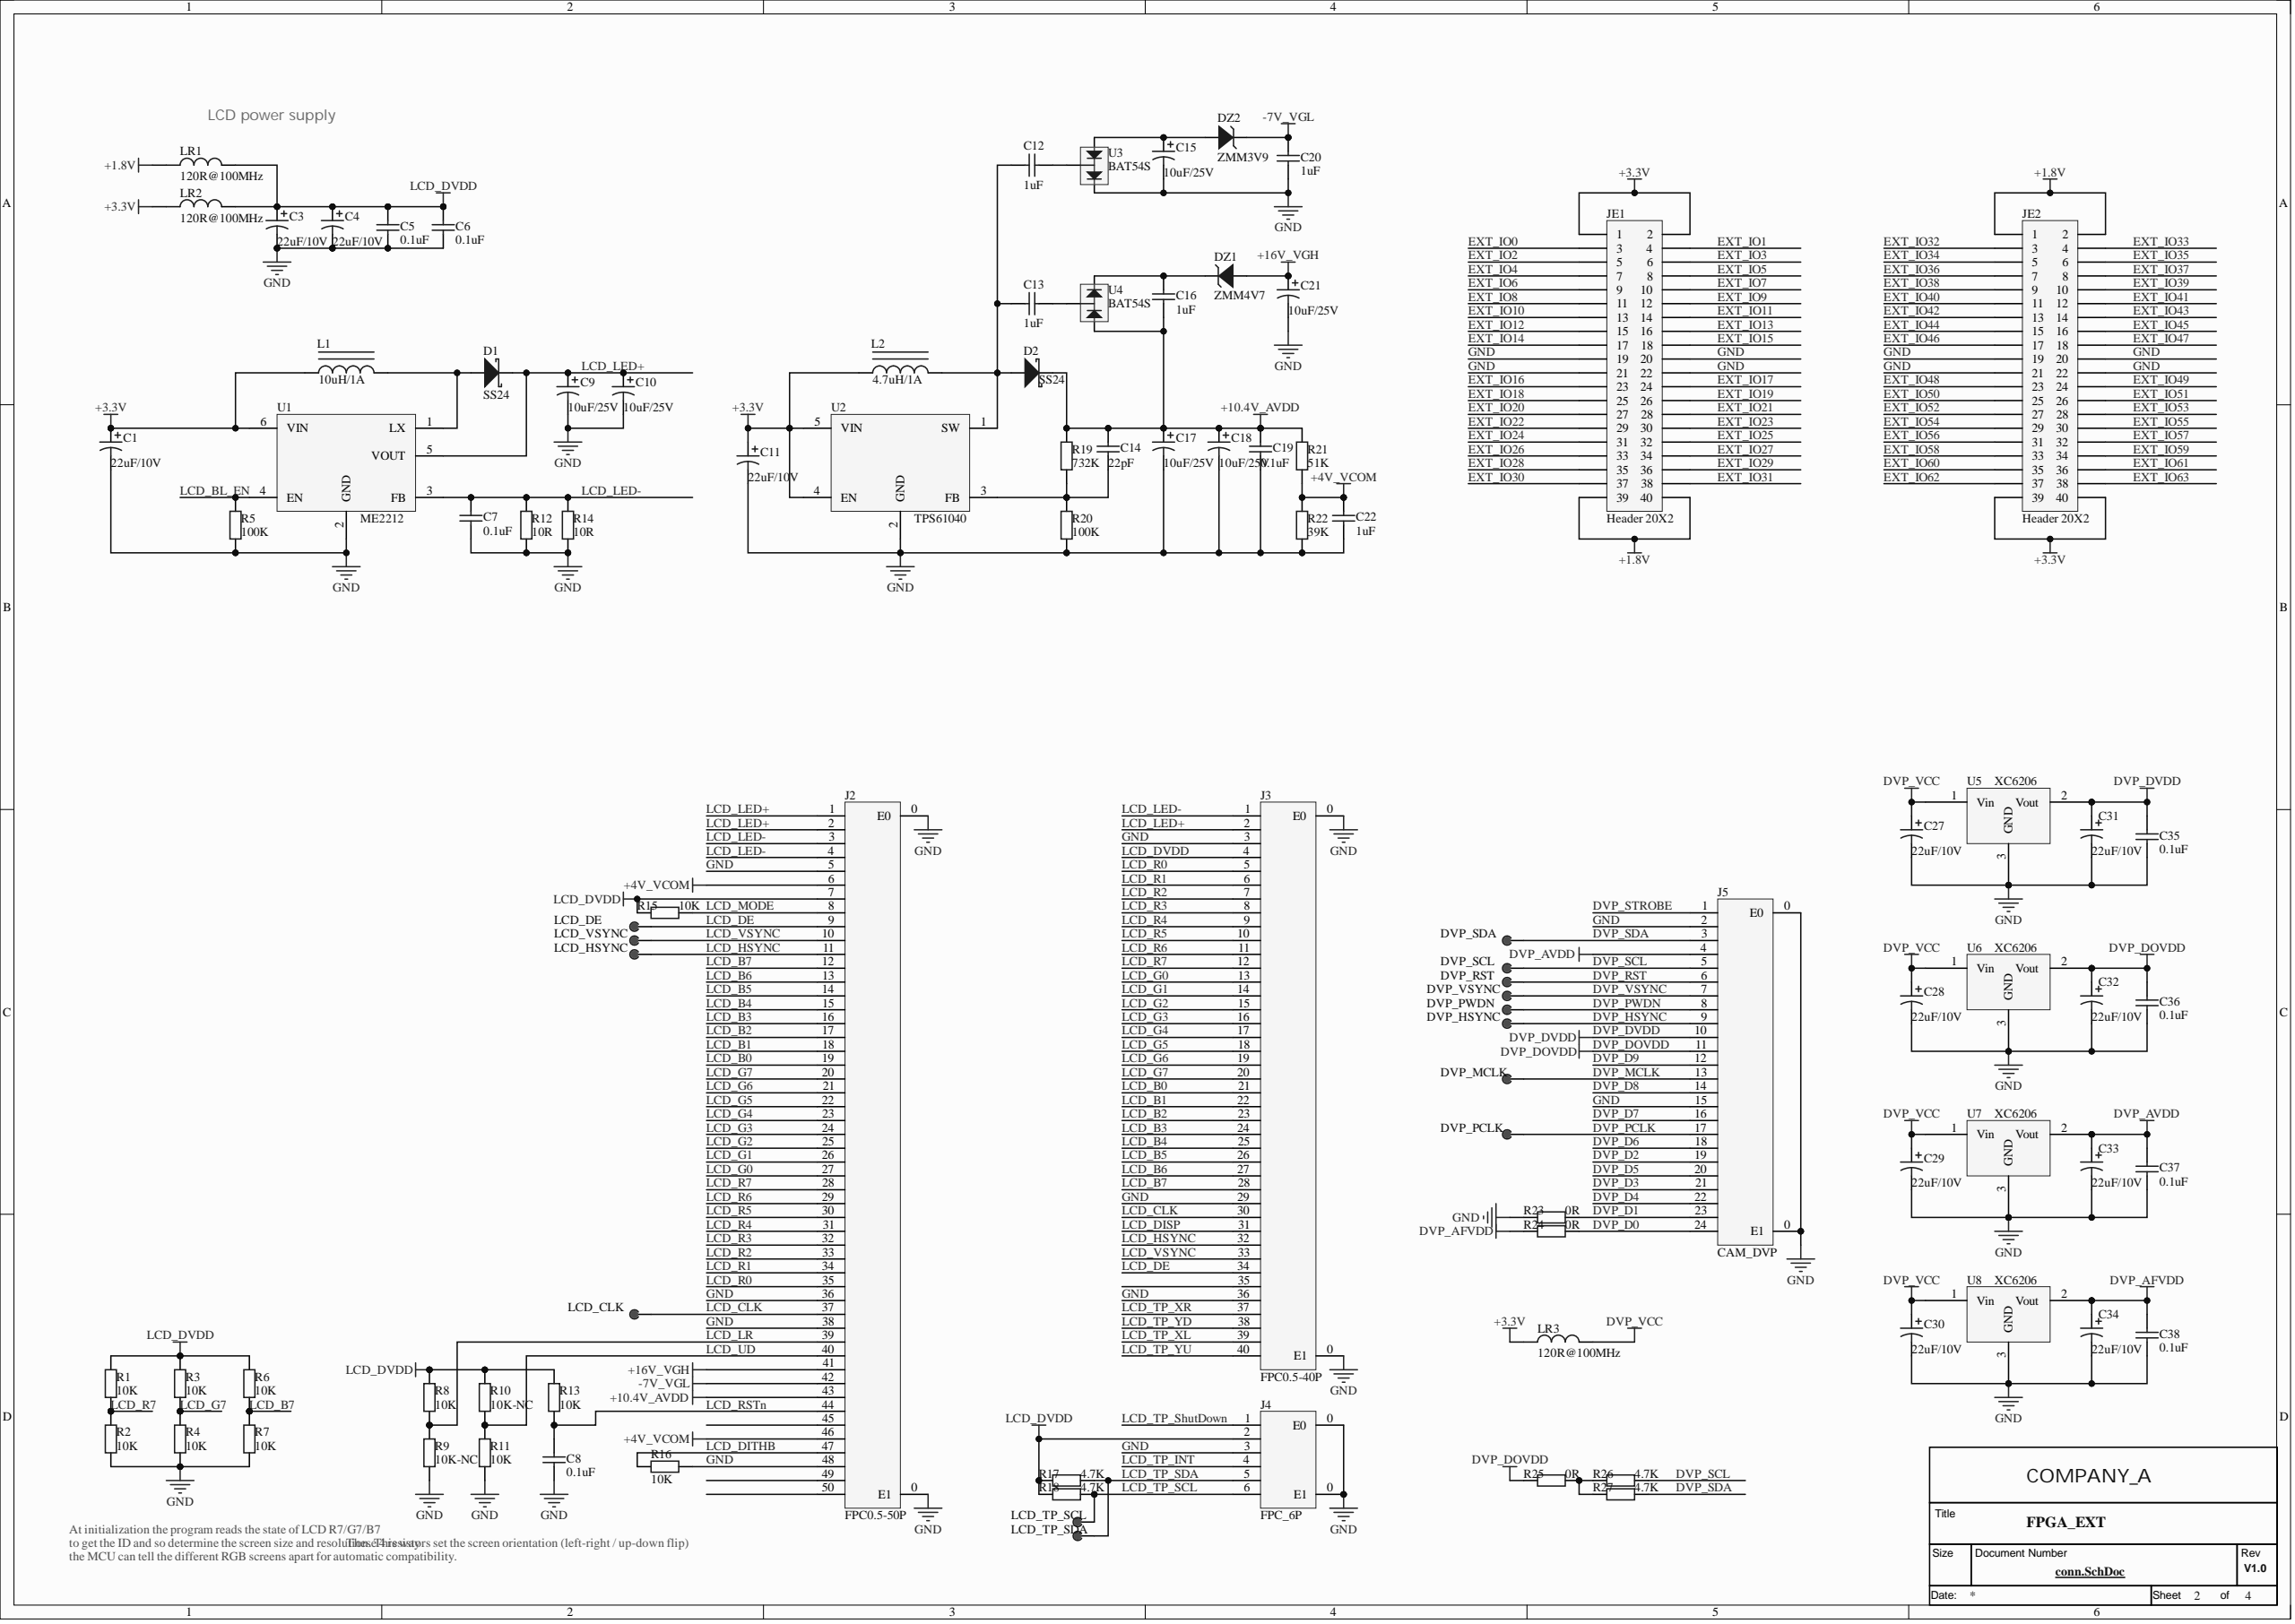Circuit board | Altium Designer | 234 parts | 308 nets | one sheet of the schematic
Parts on this sheet (reference | value | footprint):
C1 | 22uF/10V | 0603C_N
C3 | 22uF/10V | 0603C_N
C5 | 0.1uF | 0603C_N
C6 | 0.1uF | 0603C_N
C8 | 0.1uF | 0603C_N
C9 | 10uF/25V | 0603C_N
C10 | 10uF/25V | 0603C_N
C11 | 22uF/10V | 0603C_N
C12 | 1uF | 0603C_N
C13 | 1uF | 0603C_N
C14 | 22pF | 0603C_N
C15 | 10uF/25V | 0603C_N
C16 | 1uF | 0603C_N
C17 | 10uF/25V | 0603C_N
C18 | 10uF/25V | 0603C_N
C19 | 0.1uF | 0603C_N
C20 | 1uF | 0603C_N
C21 | 10uF/25V | 0603C_N
C22 | 1uF | 0603C_N
C27 | 22uF/10V | 0603C_N
C28 | 22uF/10V | 0603C_N
C29 | 22uF/10V | 0603C_N
C30 | 22uF/10V | 0603C_N
C31 | 22uF/10V | 0603C_N
C32 | 22uF/10V | 0603C_N
C33 | 22uF/10V | 0603C_N
C34 | 22uF/10V | 0603C_N
C35 | 0.1uF | 0603C_N
C36 | 0.1uF | 0603C_N
C37 | 0.1uF | 0603C_N
C38 | 0.1uF | 0603C_N
D1 | SS24 | DO-214AC
D2 | SS24 | DO-214AC
DZ1 | ZMM4V7 | LL-34
DZ2 | ZMM3V9 | LL-34
J2 | FPC0.5-50P | FPC0.5-50P
J3 | FPC0.5-40P | FPC0.5-40P
J4 | FPC_6P | FPC0.5-6P
J5 | CAM_DVP | FPC0.5-24P
JE1 | Header 20X2 | HDR2X20
JE2 | Header 20X2 | HDR2X20
L1 | 10uH/1A | LD-5.5mm
L2 | 4.7uH/1A | LD-5.5mm
LR1 | 120R@100MHz | 0603R_N
LR2 | 120R@100MHz | 0603R_N
LR3 | 120R@100MHz | 0603R_N
R1 | 10K | 0603R_N
R2 | 10K | 0603R_N
R3 | 10K | 0603R_N
R4 | 10K | 0603R_N
R5 | 100K | 0603R_N
R6 | 10K | 0603R_N
R7 | 10K | 0603R_N
R8 | 10K | 0603R_N
R9 | 10K-NC | 0603R_N
R10 | 10K-NC | 0603R_N
R11 | 10K | 0603R_N
R12 | 10R | 0603R_N
R13 | 10K | 0603R_N
R14 | 10R | 0603R_N
R15 | 10K | 0603R_N
R16 | 10K | 0603R_N
R17 | 4.7K | 0603R_N
R18 | 4.7K | 0603R_N
R19 | 732K | 0603R_N
R20 | 100K | 0603R_N
R21 | 51K | 0603R_N
R22 | 39K | 0603R_N
R23 | 0R | 0603R_N
R24 | 0R | 0603R_N
R25 | 0R | 0603R_N
R26 | 4.7K | 0603R_N
R27 | 4.7K | 0603R_N
U1 | ME2212 | SOT-23-6
U2 | TPS61040 | SOT-23-5
U3 | BAT54S | SOT-23
U4 | BAT54S | SOT-23
U5 | XC6206 | SOT-23
U6 | XC6206 | SOT-23
U7 | XC6206 | SOT-23
U8 | XC6206 | SOT-23
Nets of these parts (net: part-pin ...):
NetR25_2: R25-2 R26-2 R27-2
NetD1_1: D1-1 L1-2 U1-1
NetC16_1: C16-1 DZ1-2 U4-2
NetC15_1: C15-1 DZ2-1 U3-1
NetC14_1: C14-1 R19-1 R20-2 U2-3
NetC13_1: C13-1 U4-3
NetC12_2: C12-2 C13-2 D2-1 L2-2 U2-1
NetC12_1: C12-1 U3-3
LCD_VSYNC: J2-10 J3-33
LCD_UD: R10-1 R11-2 J2-40
LCD_TP_SDA: J4-5 R17-1
LCD_TP_SCL: J4-6 R18-1
LCD_TP_INT: J4-4
LCD_RSTn: C8-2 R13-1 J2-44
LCD_R7: R1-1 R2-2 J2-28 J3-12
LCD_R6: J2-29 J3-11
LCD_R5: J2-30 J3-10
LCD_R4: J2-31 J3-9
LCD_R3: J2-32 J3-8
LCD_R2: J2-33 J3-7
LCD_R1: J2-34 J3-6
LCD_R0: J2-35 J3-5
LCD_MODE: R15-1 J2-8
LCD_LR: R8-1 R9-2 J2-39
LCD_LED-: R12-2 R14-2 U1-3 J2-3 J2-4 J3-1
LCD_LED+: C9-1 C10-1 D1-2 U1-5 J2-1 J2-2 J3-2
LCD_HSYNC: J2-11 J3-32
LCD_G7: R3-1 R4-2 J2-20 J3-20
LCD_G6: J2-21 J3-19
LCD_G5: J2-22 J3-18
LCD_G4: J2-23 J3-17
LCD_G3: J2-24 J3-16
LCD_G2: J2-25 J3-15
LCD_G1: J2-26 J3-14
LCD_G0: J2-27 J3-13
LCD_DVDD: C3-1 C5-2 C6-2 J4-2 LR1-1 LR2-1 R1-2 R3-2 R6-2 R8-2 R10-2 R13-2 R15-2 R17-2 R18-2 J2-7 J3-4
LCD_DITHB: R16-2 J2-47
LCD_DISP: J3-31
LCD_DE: J2-9 J3-34
LCD_CLK: J2-37 J3-30
LCD_BL_EN: R5-2 U1-4
LCD_B7: R6-1 R7-2 J2-12 J3-28
LCD_B6: J2-13 J3-27
LCD_B5: J2-14 J3-26
LCD_B4: J2-15 J3-25
LCD_B3: J2-16 J3-24
LCD_B2: J2-17 J3-23
LCD_B1: J2-18 J3-22
LCD_B0: J2-19 J3-21
GND: C1-2 C3-2 C5-1 C6-1 C8-1 C9-2 C10-2 C11-2 C15-2 C17-2 C18-2 C19-1 C20-2 C21-2 C22-2 C27-2 C28-2 C29-2 C30-2 C31-2 C32-2 C33-2 C34-2 C35-1 C36-1 C37-1 C38-1 J4-0 J4-3 R2-1 R4-1 R5-1 R7-1 R9-1 R11-1 R12-1 R14-1 R16-1 R20-1 R22-1 R23-1 U1-2 U2-2 U3-2 U5-3 U6-3 U7-3 U8-3 J2-0 J2-5 J2-36 J2-38 J2-48 J3-0 J3-3 J3-29 J3-36 J5-0 J5-2 J5-15 JE1-19 JE1-20 JE1-21 JE1-22 JE2-19 JE2-20 JE2-21 JE2-22
EXT_IO63: JE2-38
EXT_IO62: JE2-37
EXT_IO61: JE2-36
EXT_IO60: JE2-35
EXT_IO59: JE2-34
EXT_IO58: JE2-33
EXT_IO57: JE2-32
EXT_IO56: JE2-31
EXT_IO55: JE2-30
EXT_IO54: JE2-29
EXT_IO53: JE2-28
EXT_IO52: JE2-27
EXT_IO51: JE2-26
EXT_IO50: JE2-25
EXT_IO49: JE2-24
EXT_IO48: JE2-23
EXT_IO47: JE2-18
EXT_IO46: JE2-17
EXT_IO45: JE2-16
EXT_IO44: JE2-15
EXT_IO43: JE2-14
EXT_IO42: JE2-13
EXT_IO41: JE2-12
EXT_IO40: JE2-11
EXT_IO39: JE2-10
EXT_IO38: JE2-9
EXT_IO37: JE2-8
EXT_IO36: JE2-7
EXT_IO35: JE2-6
EXT_IO34: JE2-5
EXT_IO33: JE2-4
EXT_IO32: JE2-3
EXT_IO31: JE1-38
EXT_IO30: JE1-37
EXT_IO29: JE1-36
EXT_IO28: JE1-35
EXT_IO27: JE1-34
EXT_IO26: JE1-33
EXT_IO25: JE1-32
EXT_IO24: JE1-31
EXT_IO23: JE1-30
EXT_IO22: JE1-29
EXT_IO21: JE1-28
EXT_IO20: JE1-27
EXT_IO19: JE1-26
EXT_IO18: JE1-25
EXT_IO17: JE1-24
EXT_IO16: JE1-23
EXT_IO15: JE1-18
EXT_IO14: JE1-17
EXT_IO13: JE1-16
EXT_IO12: JE1-15
EXT_IO11: JE1-14
EXT_IO10: JE1-13
EXT_IO9: JE1-12
EXT_IO8: JE1-11
EXT_IO7: JE1-10
EXT_IO6: JE1-9
EXT_IO5: JE1-8
EXT_IO4: JE1-7
EXT_IO3: JE1-6
EXT_IO2: JE1-5
EXT_IO1: JE1-4
EXT_IO0: JE1-3
DVP_VSYNC: J5-7
DVP_VCC: C27-1 C28-1 C29-1 C30-1 LR3-1 U5-1 U6-1 U7-1 U8-1
DVP_STROBE: J5-1
DVP_SDA: R27-1 J5-3
DVP_SCL: R26-1 J5-5
DVP_RST: J5-6
DVP_PWDN: J5-8
DVP_PCLK: J5-17
DVP_MCLK: J5-13
DVP_HSYNC: J5-9
DVP_DVDD: C31-1 C35-2 U5-2 J5-10
DVP_DOVDD: C32-1 C36-2 R25-1 U6-2 J5-11
DVP_D9: J5-12
DVP_D8: J5-14
DVP_D7: J5-16
DVP_D6: J5-18
DVP_D5: J5-20
DVP_D4: J5-22
DVP_D3: J5-21
DVP_D2: J5-19
DVP_D1: R23-2 J5-23
DVP_D0: R24-2 J5-24
DVP_AVDD: C33-1 C37-2 U7-2 J5-4
DVP_AFVDD: C34-1 C38-2 R24-1 U8-2
-7V_VGL: C20-1 DZ2-2 J2-42
+16V_VGH: C21-1 DZ1-1 J2-41
+10.4V_AVDD: C14-2 C16-2 C17-1 C18-1 C19-2 D2-2 R19-2 R21-2 U4-1 J2-43
+4V_VCOM: C22-1 R21-1 R22-2 J2-6 J2-46
+3.3V: C1-1 C11-1 L1-1 L2-1 LR2-2 LR3-2 U1-6 U2-4 U2-5 JE1-1 JE1-2 JE2-39 JE2-40
+1.8V: LR1-2 JE1-39 JE1-40 JE2-1 JE2-2